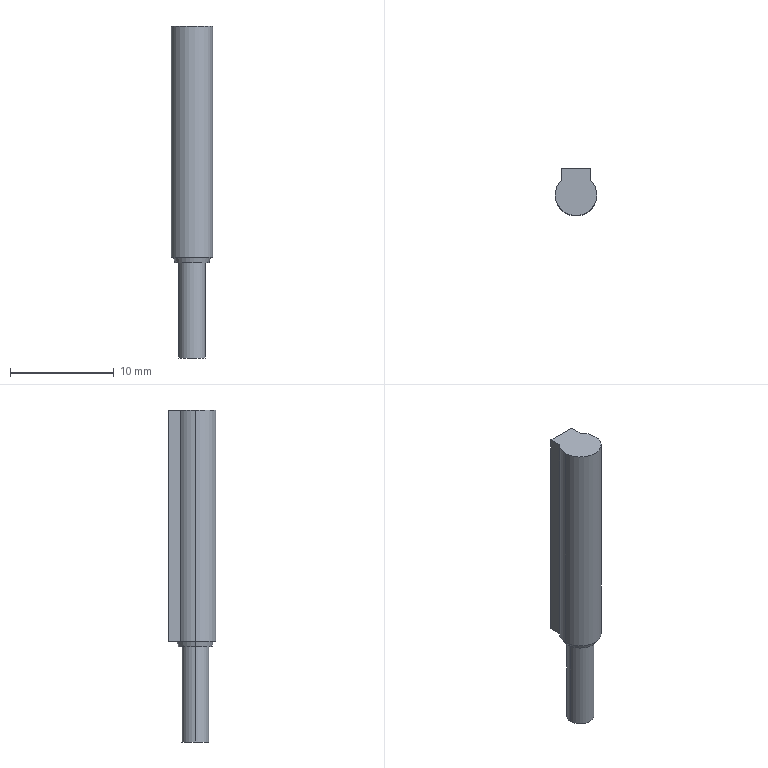Part | SolidWorks | features BaseBody 1 | 1 solid | 24 faces | box 4 x 4.6 x 32 mm | volume 381.799 mm3 | plane 12 | cylinder 10 | cone 2 | commonest cylinder face diameters 2.1 x3 4 x3 2.5 x2 2.6 x2
STEP:
#1=CARTESIAN_POINT('',(-1.4,1.428,-22.3));
#2=VERTEX_POINT('',#1);
#3=CARTESIAN_POINT('',(-2.,0.,-22.3));
#4=VERTEX_POINT('',#3);
#5=CARTESIAN_POINT('',(0.,0.,-22.3));
#6=DIRECTION('',(0.,0.,1.));
#7=DIRECTION('',(1.,0.,0.));
#8=AXIS2_PLACEMENT_3D('',#5,#6,#7);
#9=CIRCLE('',#8,2.);
#10=EDGE_CURVE('',#2,#4,#9,.T.);
#11=ORIENTED_EDGE('',*,*,#10,.T.);
#12=CARTESIAN_POINT('',(-2.,0.,0.));
#13=VERTEX_POINT('',#12);
#14=CARTESIAN_POINT('',(-2.,0.,-22.3));
#15=DIRECTION('',(0.,0.,1.));
#16=VECTOR('',#15,1000.);
#17=LINE('',#14,#16);
#18=EDGE_CURVE('',#4,#13,#17,.T.);
#19=ORIENTED_EDGE('',*,*,#18,.T.);
#20=CARTESIAN_POINT('',(-1.4,1.428,0.));
#21=VERTEX_POINT('',#20);
#22=CARTESIAN_POINT('',(0.,0.,0.));
#23=DIRECTION('',(0.,0.,-1.));
#24=DIRECTION('',(1.,0.,0.));
#25=AXIS2_PLACEMENT_3D('',#22,#23,#24);
#26=CIRCLE('',#25,2.);
#27=EDGE_CURVE('',#13,#21,#26,.T.);
#28=ORIENTED_EDGE('',*,*,#27,.T.);
#29=CARTESIAN_POINT('',(-1.4,1.428,-22.3));
#30=DIRECTION('',(0.,0.,-1.));
#31=VECTOR('',#30,1000.);
#32=LINE('',#29,#31);
#33=EDGE_CURVE('',#21,#2,#32,.T.);
#34=ORIENTED_EDGE('',*,*,#33,.T.);
#35=EDGE_LOOP('',(#11,#19,#28,#34));
#36=FACE_OUTER_BOUND('',#35,.T.);
#37=CARTESIAN_POINT('',(0.,0.,-22.3));
#38=DIRECTION('',(0.,0.,1.));
#39=DIRECTION('',(1.,0.,0.));
#40=AXIS2_PLACEMENT_3D('',#37,#38,#39);
#41=CYLINDRICAL_SURFACE('',#40,2.);
#42=ADVANCED_FACE('',(#36),#41,.T.);
#43=ORIENTED_EDGE('',*,*,#18,.F.);
#44=CARTESIAN_POINT('',(2.,0.,-22.3));
#45=VERTEX_POINT('',#44);
#46=CARTESIAN_POINT('',(0.,0.,-22.3));
#47=DIRECTION('',(0.,0.,1.));
#48=DIRECTION('',(1.,0.,0.));
#49=AXIS2_PLACEMENT_3D('',#46,#47,#48);
#50=CIRCLE('',#49,2.);
#51=EDGE_CURVE('',#4,#45,#50,.T.);
#52=ORIENTED_EDGE('',*,*,#51,.T.);
#53=CARTESIAN_POINT('',(2.,0.,0.));
#54=VERTEX_POINT('',#53);
#55=CARTESIAN_POINT('',(2.,0.,-22.3));
#56=DIRECTION('',(0.,0.,1.));
#57=VECTOR('',#56,1000.);
#58=LINE('',#55,#57);
#59=EDGE_CURVE('',#45,#54,#58,.T.);
#60=ORIENTED_EDGE('',*,*,#59,.T.);
#61=CARTESIAN_POINT('',(0.,0.,0.));
#62=DIRECTION('',(0.,0.,-1.));
#63=DIRECTION('',(1.,0.,0.));
#64=AXIS2_PLACEMENT_3D('',#61,#62,#63);
#65=CIRCLE('',#64,2.);
#66=EDGE_CURVE('',#54,#13,#65,.T.);
#67=ORIENTED_EDGE('',*,*,#66,.T.);
#68=EDGE_LOOP('',(#43,#52,#60,#67));
#69=FACE_OUTER_BOUND('',#68,.T.);
#70=CARTESIAN_POINT('',(0.,0.,-22.3));
#71=DIRECTION('',(0.,0.,1.));
#72=DIRECTION('',(1.,0.,0.));
#73=AXIS2_PLACEMENT_3D('',#70,#71,#72);
#74=CYLINDRICAL_SURFACE('',#73,2.);
#75=ADVANCED_FACE('',(#69),#74,.T.);
#76=CARTESIAN_POINT('',(1.65,0.,-22.8));
#77=VERTEX_POINT('',#76);
#78=CARTESIAN_POINT('',(-1.65,0.,-22.8));
#79=VERTEX_POINT('',#78);
#80=CARTESIAN_POINT('',(0.,0.,-22.8));
#81=DIRECTION('',(0.,0.,1.));
#82=DIRECTION('',(1.,0.,0.));
#83=AXIS2_PLACEMENT_3D('',#80,#81,#82);
#84=CIRCLE('',#83,1.65);
#85=EDGE_CURVE('',#77,#79,#84,.T.);
#86=ORIENTED_EDGE('',*,*,#85,.T.);
#87=CARTESIAN_POINT('',(-1.784,0.,-22.3));
#88=VERTEX_POINT('',#87);
#89=CARTESIAN_POINT('',(-1.784,0.,-22.3));
#90=DIRECTION('',(-0.2588,0.,0.9659));
#91=VECTOR('',#90,1000.);
#92=LINE('',#89,#91);
#93=EDGE_CURVE('',#79,#88,#92,.T.);
#94=ORIENTED_EDGE('',*,*,#93,.T.);
#95=CARTESIAN_POINT('',(1.784,0.,-22.3));
#96=VERTEX_POINT('',#95);
#97=CARTESIAN_POINT('',(0.,0.,-22.3));
#98=DIRECTION('',(0.,0.,-1.));
#99=DIRECTION('',(1.,0.,0.));
#100=AXIS2_PLACEMENT_3D('',#97,#98,#99);
#101=CIRCLE('',#100,1.784);
#102=EDGE_CURVE('',#88,#96,#101,.T.);
#103=ORIENTED_EDGE('',*,*,#102,.T.);
#104=CARTESIAN_POINT('',(1.784,0.,-22.3));
#105=DIRECTION('',(0.2588,0.,0.9659));
#106=VECTOR('',#105,1000.);
#107=LINE('',#104,#106);
#108=EDGE_CURVE('',#77,#96,#107,.T.);
#109=ORIENTED_EDGE('',*,*,#108,.F.);
#110=EDGE_LOOP('',(#86,#94,#103,#109));
#111=FACE_OUTER_BOUND('',#110,.T.);
#112=CARTESIAN_POINT('',(0.,0.,-22.3));
#113=DIRECTION('',(0.,0.,1.));
#114=DIRECTION('',(1.,0.,0.));
#115=AXIS2_PLACEMENT_3D('',#112,#113,#114);
#116=CONICAL_SURFACE('',#115,1.784,0.2618);
#117=ADVANCED_FACE('',(#111),#116,.T.);
#118=CARTESIAN_POINT('',(0.,2.4,-3.25));
#119=VERTEX_POINT('',#118);
#120=CARTESIAN_POINT('',(0.,2.4,-0.75));
#121=VERTEX_POINT('',#120);
#122=CARTESIAN_POINT('',(0.,2.4,-2.));
#123=DIRECTION('',(0.,1.,0.));
#124=DIRECTION('',(0.,0.,1.));
#125=AXIS2_PLACEMENT_3D('',#122,#123,#124);
#126=CIRCLE('',#125,1.25);
#127=EDGE_CURVE('',#119,#121,#126,.T.);
#128=ORIENTED_EDGE('',*,*,#127,.F.);
#129=CARTESIAN_POINT('',(0.,2.6,-3.25));
#130=VERTEX_POINT('',#129);
#131=CARTESIAN_POINT('',(0.,2.4,-3.25));
#132=DIRECTION('',(0.,1.,0.));
#133=VECTOR('',#132,1000.);
#134=LINE('',#131,#133);
#135=EDGE_CURVE('',#119,#130,#134,.T.);
#136=ORIENTED_EDGE('',*,*,#135,.T.);
#137=CARTESIAN_POINT('',(0.,2.6,-0.75));
#138=VERTEX_POINT('',#137);
#139=CARTESIAN_POINT('',(0.,2.6,-2.));
#140=DIRECTION('',(0.,-1.,0.));
#141=DIRECTION('',(0.,0.,1.));
#142=AXIS2_PLACEMENT_3D('',#139,#140,#141);
#143=CIRCLE('',#142,1.25);
#144=EDGE_CURVE('',#138,#130,#143,.T.);
#145=ORIENTED_EDGE('',*,*,#144,.F.);
#146=CARTESIAN_POINT('',(0.,2.4,-0.75));
#147=DIRECTION('',(0.,1.,0.));
#148=VECTOR('',#147,1000.);
#149=LINE('',#146,#148);
#150=EDGE_CURVE('',#121,#138,#149,.T.);
#151=ORIENTED_EDGE('',*,*,#150,.F.);
#152=EDGE_LOOP('',(#128,#136,#145,#151));
#153=FACE_OUTER_BOUND('',#152,.T.);
#154=CARTESIAN_POINT('',(0.,2.4,-2.));
#155=DIRECTION('',(0.,1.,0.));
#156=DIRECTION('',(0.,0.,1.));
#157=AXIS2_PLACEMENT_3D('',#154,#155,#156);
#158=CYLINDRICAL_SURFACE('',#157,1.25);
#159=ADVANCED_FACE('',(#153),#158,.F.);
#160=CARTESIAN_POINT('',(1.3,0.,-32.));
#161=VERTEX_POINT('',#160);
#162=CARTESIAN_POINT('',(-1.3,0.,-32.));
#163=VERTEX_POINT('',#162);
#164=CARTESIAN_POINT('',(0.,0.,-32.));
#165=DIRECTION('',(0.,0.,1.));
#166=DIRECTION('',(1.,0.,0.));
#167=AXIS2_PLACEMENT_3D('',#164,#165,#166);
#168=CIRCLE('',#167,1.3);
#169=EDGE_CURVE('',#161,#163,#168,.T.);
#170=ORIENTED_EDGE('',*,*,#169,.T.);
#171=CARTESIAN_POINT('',(-1.3,0.,-22.8));
#172=VERTEX_POINT('',#171);
#173=CARTESIAN_POINT('',(-1.3,0.,-32.));
#174=DIRECTION('',(0.,0.,1.));
#175=VECTOR('',#174,1000.);
#176=LINE('',#173,#175);
#177=EDGE_CURVE('',#163,#172,#176,.T.);
#178=ORIENTED_EDGE('',*,*,#177,.T.);
#179=CARTESIAN_POINT('',(1.3,0.,-22.8));
#180=VERTEX_POINT('',#179);
#181=CARTESIAN_POINT('',(0.,0.,-22.8));
#182=DIRECTION('',(0.,0.,-1.));
#183=DIRECTION('',(1.,0.,0.));
#184=AXIS2_PLACEMENT_3D('',#181,#182,#183);
#185=CIRCLE('',#184,1.3);
#186=EDGE_CURVE('',#172,#180,#185,.T.);
#187=ORIENTED_EDGE('',*,*,#186,.T.);
#188=CARTESIAN_POINT('',(1.3,0.,-32.));
#189=DIRECTION('',(0.,0.,1.));
#190=VECTOR('',#189,1000.);
#191=LINE('',#188,#190);
#192=EDGE_CURVE('',#161,#180,#191,.T.);
#193=ORIENTED_EDGE('',*,*,#192,.F.);
#194=EDGE_LOOP('',(#170,#178,#187,#193));
#195=FACE_OUTER_BOUND('',#194,.T.);
#196=CARTESIAN_POINT('',(0.,0.,-32.));
#197=DIRECTION('',(0.,0.,1.));
#198=DIRECTION('',(1.,0.,0.));
#199=AXIS2_PLACEMENT_3D('',#196,#197,#198);
#200=CYLINDRICAL_SURFACE('',#199,1.3);
#201=ADVANCED_FACE('',(#195),#200,.T.);
#202=CARTESIAN_POINT('',(0.,2.4,-0.95));
#203=VERTEX_POINT('',#202);
#204=CARTESIAN_POINT('',(-0.5443,2.4,-1.102));
#205=VERTEX_POINT('',#204);
#206=CARTESIAN_POINT('',(0.,2.4,-2.));
#207=DIRECTION('',(0.,-1.,0.));
#208=DIRECTION('',(0.,0.,1.));
#209=AXIS2_PLACEMENT_3D('',#206,#207,#208);
#210=CIRCLE('',#209,1.05);
#211=EDGE_CURVE('',#203,#205,#210,.T.);
#212=ORIENTED_EDGE('',*,*,#211,.F.);
#213=CARTESIAN_POINT('',(0.,2.6,-0.95));
#214=VERTEX_POINT('',#213);
#215=CARTESIAN_POINT('',(0.,2.4,-0.95));
#216=DIRECTION('',(0.,1.,0.));
#217=VECTOR('',#216,1000.);
#218=LINE('',#215,#217);
#219=EDGE_CURVE('',#203,#214,#218,.T.);
#220=ORIENTED_EDGE('',*,*,#219,.T.);
#221=CARTESIAN_POINT('',(-0.5443,2.6,-1.102));
#222=VERTEX_POINT('',#221);
#223=CARTESIAN_POINT('',(0.,2.6,-2.));
#224=DIRECTION('',(0.,-1.,0.));
#225=DIRECTION('',(0.,0.,1.));
#226=AXIS2_PLACEMENT_3D('',#223,#224,#225);
#227=CIRCLE('',#226,1.05);
#228=EDGE_CURVE('',#214,#222,#227,.T.);
#229=ORIENTED_EDGE('',*,*,#228,.T.);
#230=CARTESIAN_POINT('',(-0.5443,2.4,-1.102));
#231=DIRECTION('',(0.,-1.,0.));
#232=VECTOR('',#231,1000.);
#233=LINE('',#230,#232);
#234=EDGE_CURVE('',#222,#205,#233,.T.);
#235=ORIENTED_EDGE('',*,*,#234,.T.);
#236=EDGE_LOOP('',(#212,#220,#229,#235));
#237=FACE_OUTER_BOUND('',#236,.T.);
#238=CARTESIAN_POINT('',(0.,2.4,-2.));
#239=DIRECTION('',(0.,1.,0.));
#240=DIRECTION('',(0.,0.,1.));
#241=AXIS2_PLACEMENT_3D('',#238,#239,#240);
#242=CYLINDRICAL_SURFACE('',#241,1.05);
#243=ADVANCED_FACE('',(#237),#242,.T.);
#244=ORIENTED_EDGE('',*,*,#59,.F.);
#245=CARTESIAN_POINT('',(1.4,1.428,-22.3));
#246=VERTEX_POINT('',#245);
#247=CARTESIAN_POINT('',(0.,0.,-22.3));
#248=DIRECTION('',(0.,0.,1.));
#249=DIRECTION('',(1.,0.,0.));
#250=AXIS2_PLACEMENT_3D('',#247,#248,#249);
#251=CIRCLE('',#250,2.);
#252=EDGE_CURVE('',#45,#246,#251,.T.);
#253=ORIENTED_EDGE('',*,*,#252,.T.);
#254=CARTESIAN_POINT('',(1.4,1.428,0.));
#255=VERTEX_POINT('',#254);
#256=CARTESIAN_POINT('',(1.4,1.428,-22.3));
#257=DIRECTION('',(0.,0.,1.));
#258=VECTOR('',#257,1000.);
#259=LINE('',#256,#258);
#260=EDGE_CURVE('',#246,#255,#259,.T.);
#261=ORIENTED_EDGE('',*,*,#260,.T.);
#262=CARTESIAN_POINT('',(0.,0.,0.));
#263=DIRECTION('',(0.,0.,-1.));
#264=DIRECTION('',(1.,0.,0.));
#265=AXIS2_PLACEMENT_3D('',#262,#263,#264);
#266=CIRCLE('',#265,2.);
#267=EDGE_CURVE('',#255,#54,#266,.T.);
#268=ORIENTED_EDGE('',*,*,#267,.T.);
#269=EDGE_LOOP('',(#244,#253,#261,#268));
#270=FACE_OUTER_BOUND('',#269,.T.);
#271=CARTESIAN_POINT('',(0.,0.,-22.3));
#272=DIRECTION('',(0.,0.,1.));
#273=DIRECTION('',(1.,0.,0.));
#274=AXIS2_PLACEMENT_3D('',#271,#272,#273);
#275=CYLINDRICAL_SURFACE('',#274,2.);
#276=ADVANCED_FACE('',(#270),#275,.T.);
#277=CARTESIAN_POINT('',(1.4,2.6,-22.3));
#278=VERTEX_POINT('',#277);
#279=CARTESIAN_POINT('',(1.4,1.428,-22.3));
#280=DIRECTION('',(0.,1.,0.));
#281=VECTOR('',#280,1000.);
#282=LINE('',#279,#281);
#283=EDGE_CURVE('',#246,#278,#282,.T.);
#284=ORIENTED_EDGE('',*,*,#283,.T.);
#285=CARTESIAN_POINT('',(1.4,2.6,0.));
#286=VERTEX_POINT('',#285);
#287=CARTESIAN_POINT('',(1.4,2.6,-22.3));
#288=DIRECTION('',(0.,0.,1.));
#289=VECTOR('',#288,1000.);
#290=LINE('',#287,#289);
#291=EDGE_CURVE('',#278,#286,#290,.T.);
#292=ORIENTED_EDGE('',*,*,#291,.T.);
#293=CARTESIAN_POINT('',(1.4,1.428,0.));
#294=DIRECTION('',(0.,-1.,0.));
#295=VECTOR('',#294,1000.);
#296=LINE('',#293,#295);
#297=EDGE_CURVE('',#286,#255,#296,.T.);
#298=ORIENTED_EDGE('',*,*,#297,.T.);
#299=ORIENTED_EDGE('',*,*,#260,.F.);
#300=EDGE_LOOP('',(#284,#292,#298,#299));
#301=FACE_OUTER_BOUND('',#300,.T.);
#302=CARTESIAN_POINT('',(1.4,1.428,-22.3));
#303=DIRECTION('',(1.,0.,0.));
#304=DIRECTION('',(0.,1.,0.));
#305=AXIS2_PLACEMENT_3D('',#302,#303,#304);
#306=PLANE('',#305);
#307=ADVANCED_FACE('',(#301),#306,.T.);
#308=CARTESIAN_POINT('',(-1.4,2.6,-22.3));
#309=VERTEX_POINT('',#308);
#310=CARTESIAN_POINT('',(0.,2.6,-22.3));
#311=DIRECTION('',(-1.,0.,0.));
#312=VECTOR('',#311,1000.);
#313=LINE('',#310,#312);
#314=EDGE_CURVE('',#278,#309,#313,.T.);
#315=ORIENTED_EDGE('',*,*,#314,.F.);
#316=ORIENTED_EDGE('',*,*,#283,.F.);
#317=ORIENTED_EDGE('',*,*,#252,.F.);
#318=ORIENTED_EDGE('',*,*,#51,.F.);
#319=ORIENTED_EDGE('',*,*,#10,.F.);
#320=CARTESIAN_POINT('',(-1.4,0.,-22.3));
#321=DIRECTION('',(0.,-1.,0.));
#322=VECTOR('',#321,1000.);
#323=LINE('',#320,#322);
#324=EDGE_CURVE('',#309,#2,#323,.T.);
#325=ORIENTED_EDGE('',*,*,#324,.F.);
#326=EDGE_LOOP('',(#315,#316,#317,#318,#319,#325));
#327=FACE_OUTER_BOUND('',#326,.T.);
#328=CARTESIAN_POINT('',(0.,0.,-22.3));
#329=DIRECTION('',(0.,0.,-1.));
#330=DIRECTION('',(1.,0.,0.));
#331=AXIS2_PLACEMENT_3D('',#328,#329,#330);
#332=CIRCLE('',#331,1.784);
#333=EDGE_CURVE('',#96,#88,#332,.T.);
#334=ORIENTED_EDGE('',*,*,#333,.F.);
#335=ORIENTED_EDGE('',*,*,#102,.F.);
#336=EDGE_LOOP('',(#334,#335));
#337=FACE_BOUND('',#336,.T.);
#338=CARTESIAN_POINT('',(0.,0.,-22.3));
#339=DIRECTION('',(0.,0.,1.));
#340=DIRECTION('',(1.,0.,0.));
#341=AXIS2_PLACEMENT_3D('',#338,#339,#340);
#342=PLANE('',#341);
#343=ADVANCED_FACE('',(#327,#337),#342,.F.);
#344=ORIENTED_EDGE('',*,*,#324,.T.);
#345=ORIENTED_EDGE('',*,*,#33,.F.);
#346=CARTESIAN_POINT('',(-1.4,2.6,0.));
#347=VERTEX_POINT('',#346);
#348=CARTESIAN_POINT('',(-1.4,2.6,0.));
#349=DIRECTION('',(0.,1.,0.));
#350=VECTOR('',#349,1000.);
#351=LINE('',#348,#350);
#352=EDGE_CURVE('',#21,#347,#351,.T.);
#353=ORIENTED_EDGE('',*,*,#352,.T.);
#354=CARTESIAN_POINT('',(-1.4,2.6,-22.3));
#355=DIRECTION('',(0.,0.,-1.));
#356=VECTOR('',#355,1000.);
#357=LINE('',#354,#356);
#358=EDGE_CURVE('',#347,#309,#357,.T.);
#359=ORIENTED_EDGE('',*,*,#358,.T.);
#360=EDGE_LOOP('',(#344,#345,#353,#359));
#361=FACE_OUTER_BOUND('',#360,.T.);
#362=CARTESIAN_POINT('',(-1.4,2.6,-22.3));
#363=DIRECTION('',(-1.,0.,0.));
#364=DIRECTION('',(0.,-1.,0.));
#365=AXIS2_PLACEMENT_3D('',#362,#363,#364);
#366=PLANE('',#365);
#367=ADVANCED_FACE('',(#361),#366,.T.);
#368=ORIENTED_EDGE('',*,*,#297,.F.);
#369=CARTESIAN_POINT('',(0.,2.6,0.));
#370=DIRECTION('',(-1.,0.,0.));
#371=VECTOR('',#370,1000.);
#372=LINE('',#369,#371);
#373=EDGE_CURVE('',#286,#347,#372,.T.);
#374=ORIENTED_EDGE('',*,*,#373,.T.);
#375=ORIENTED_EDGE('',*,*,#352,.F.);
#376=ORIENTED_EDGE('',*,*,#27,.F.);
#377=ORIENTED_EDGE('',*,*,#66,.F.);
#378=ORIENTED_EDGE('',*,*,#267,.F.);
#379=EDGE_LOOP('',(#368,#374,#375,#376,#377,#378));
#380=FACE_OUTER_BOUND('',#379,.T.);
#381=CARTESIAN_POINT('',(0.,0.,0.));
#382=DIRECTION('',(0.,0.,1.));
#383=DIRECTION('',(1.,0.,0.));
#384=AXIS2_PLACEMENT_3D('',#381,#382,#383);
#385=PLANE('',#384);
#386=ADVANCED_FACE('',(#380),#385,.T.);
#387=ORIENTED_EDGE('',*,*,#314,.T.);
#388=ORIENTED_EDGE('',*,*,#358,.F.);
#389=ORIENTED_EDGE('',*,*,#373,.F.);
#390=ORIENTED_EDGE('',*,*,#291,.F.);
#391=EDGE_LOOP('',(#387,#388,#389,#390));
#392=FACE_OUTER_BOUND('',#391,.T.);
#393=ORIENTED_EDGE('',*,*,#144,.T.);
#394=CARTESIAN_POINT('',(0.,2.6,-2.));
#395=DIRECTION('',(0.,-1.,0.));
#396=DIRECTION('',(0.,0.,1.));
#397=AXIS2_PLACEMENT_3D('',#394,#395,#396);
#398=CIRCLE('',#397,1.25);
#399=EDGE_CURVE('',#130,#138,#398,.T.);
#400=ORIENTED_EDGE('',*,*,#399,.T.);
#401=EDGE_LOOP('',(#393,#400));
#402=FACE_BOUND('',#401,.T.);
#403=CARTESIAN_POINT('',(1.4,2.6,-22.3));
#404=DIRECTION('',(0.,1.,0.));
#405=DIRECTION('',(0.,0.,1.));
#406=AXIS2_PLACEMENT_3D('',#403,#404,#405);
#407=PLANE('',#406);
#408=ADVANCED_FACE('',(#392,#402),#407,.T.);
#409=ORIENTED_EDGE('',*,*,#93,.F.);
#410=CARTESIAN_POINT('',(0.,0.,-22.8));
#411=DIRECTION('',(0.,0.,1.));
#412=DIRECTION('',(1.,0.,0.));
#413=AXIS2_PLACEMENT_3D('',#410,#411,#412);
#414=CIRCLE('',#413,1.65);
#415=EDGE_CURVE('',#79,#77,#414,.T.);
#416=ORIENTED_EDGE('',*,*,#415,.T.);
#417=ORIENTED_EDGE('',*,*,#108,.T.);
#418=ORIENTED_EDGE('',*,*,#333,.T.);
#419=EDGE_LOOP('',(#409,#416,#417,#418));
#420=FACE_OUTER_BOUND('',#419,.T.);
#421=CARTESIAN_POINT('',(0.,0.,-22.3));
#422=DIRECTION('',(0.,0.,1.));
#423=DIRECTION('',(1.,0.,0.));
#424=AXIS2_PLACEMENT_3D('',#421,#422,#423);
#425=CONICAL_SURFACE('',#424,1.784,0.2618);
#426=ADVANCED_FACE('',(#420),#425,.T.);
#427=ORIENTED_EDGE('',*,*,#135,.F.);
#428=CARTESIAN_POINT('',(0.,2.4,-2.));
#429=DIRECTION('',(0.,1.,0.));
#430=DIRECTION('',(0.,0.,1.));
#431=AXIS2_PLACEMENT_3D('',#428,#429,#430);
#432=CIRCLE('',#431,1.25);
#433=EDGE_CURVE('',#121,#119,#432,.T.);
#434=ORIENTED_EDGE('',*,*,#433,.F.);
#435=ORIENTED_EDGE('',*,*,#150,.T.);
#436=ORIENTED_EDGE('',*,*,#399,.F.);
#437=EDGE_LOOP('',(#427,#434,#435,#436));
#438=FACE_OUTER_BOUND('',#437,.T.);
#439=CARTESIAN_POINT('',(0.,2.4,-2.));
#440=DIRECTION('',(0.,1.,0.));
#441=DIRECTION('',(0.,0.,1.));
#442=AXIS2_PLACEMENT_3D('',#439,#440,#441);
#443=CYLINDRICAL_SURFACE('',#442,1.25);
#444=ADVANCED_FACE('',(#438),#443,.F.);
#445=ORIENTED_EDGE('',*,*,#85,.F.);
#446=ORIENTED_EDGE('',*,*,#415,.F.);
#447=EDGE_LOOP('',(#445,#446));
#448=FACE_OUTER_BOUND('',#447,.T.);
#449=CARTESIAN_POINT('',(0.,0.,-22.8));
#450=DIRECTION('',(0.,0.,-1.));
#451=DIRECTION('',(1.,0.,0.));
#452=AXIS2_PLACEMENT_3D('',#449,#450,#451);
#453=CIRCLE('',#452,1.3);
#454=EDGE_CURVE('',#180,#172,#453,.T.);
#455=ORIENTED_EDGE('',*,*,#454,.F.);
#456=ORIENTED_EDGE('',*,*,#186,.F.);
#457=EDGE_LOOP('',(#455,#456));
#458=FACE_BOUND('',#457,.T.);
#459=CARTESIAN_POINT('',(0.,1.65,-22.8));
#460=DIRECTION('',(0.,0.,1.));
#461=DIRECTION('',(1.,0.,0.));
#462=AXIS2_PLACEMENT_3D('',#459,#460,#461);
#463=PLANE('',#462);
#464=ADVANCED_FACE('',(#448,#458),#463,.F.);
#465=ORIENTED_EDGE('',*,*,#433,.T.);
#466=ORIENTED_EDGE('',*,*,#127,.T.);
#467=EDGE_LOOP('',(#465,#466));
#468=FACE_OUTER_BOUND('',#467,.T.);
#469=CARTESIAN_POINT('',(0.8979,2.4,-2.544));
#470=VERTEX_POINT('',#469);
#471=CARTESIAN_POINT('',(-0.5443,2.4,-1.102));
#472=DIRECTION('',(0.7071,0.,-0.7071));
#473=VECTOR('',#472,1000.);
#474=LINE('',#471,#473);
#475=EDGE_CURVE('',#205,#470,#474,.T.);
#476=ORIENTED_EDGE('',*,*,#475,.T.);
#477=CARTESIAN_POINT('',(0.,2.4,-2.));
#478=DIRECTION('',(0.,-1.,0.));
#479=DIRECTION('',(0.,0.,1.));
#480=AXIS2_PLACEMENT_3D('',#477,#478,#479);
#481=CIRCLE('',#480,1.05);
#482=EDGE_CURVE('',#470,#203,#481,.T.);
#483=ORIENTED_EDGE('',*,*,#482,.T.);
#484=ORIENTED_EDGE('',*,*,#211,.T.);
#485=EDGE_LOOP('',(#476,#483,#484));
#486=FACE_BOUND('',#485,.T.);
#487=CARTESIAN_POINT('',(0.5443,2.4,-2.898));
#488=VERTEX_POINT('',#487);
#489=CARTESIAN_POINT('',(-0.8979,2.4,-1.456));
#490=VERTEX_POINT('',#489);
#491=CARTESIAN_POINT('',(0.5443,2.4,-2.898));
#492=DIRECTION('',(-0.7071,0.,0.7071));
#493=VECTOR('',#492,1000.);
#494=LINE('',#491,#493);
#495=EDGE_CURVE('',#488,#490,#494,.T.);
#496=ORIENTED_EDGE('',*,*,#495,.T.);
#497=CARTESIAN_POINT('',(0.,2.4,-2.));
#498=DIRECTION('',(0.,-1.,0.));
#499=DIRECTION('',(0.,0.,1.));
#500=AXIS2_PLACEMENT_3D('',#497,#498,#499);
#501=CIRCLE('',#500,1.05);
#502=EDGE_CURVE('',#490,#488,#501,.T.);
#503=ORIENTED_EDGE('',*,*,#502,.T.);
#504=EDGE_LOOP('',(#496,#503));
#505=FACE_BOUND('',#504,.T.);
#506=CARTESIAN_POINT('',(0.,2.4,-2.));
#507=DIRECTION('',(0.,1.,0.));
#508=DIRECTION('',(0.,0.,1.));
#509=AXIS2_PLACEMENT_3D('',#506,#507,#508);
#510=PLANE('',#509);
#511=ADVANCED_FACE('',(#468,#486,#505),#510,.T.);
#512=ORIENTED_EDGE('',*,*,#177,.F.);
#513=CARTESIAN_POINT('',(0.,0.,-32.));
#514=DIRECTION('',(0.,0.,1.));
#515=DIRECTION('',(1.,0.,0.));
#516=AXIS2_PLACEMENT_3D('',#513,#514,#515);
#517=CIRCLE('',#516,1.3);
#518=EDGE_CURVE('',#163,#161,#517,.T.);
#519=ORIENTED_EDGE('',*,*,#518,.T.);
#520=ORIENTED_EDGE('',*,*,#192,.T.);
#521=ORIENTED_EDGE('',*,*,#454,.T.);
#522=EDGE_LOOP('',(#512,#519,#520,#521));
#523=FACE_OUTER_BOUND('',#522,.T.);
#524=CARTESIAN_POINT('',(0.,0.,-32.));
#525=DIRECTION('',(0.,0.,1.));
#526=DIRECTION('',(1.,0.,0.));
#527=AXIS2_PLACEMENT_3D('',#524,#525,#526);
#528=CYLINDRICAL_SURFACE('',#527,1.3);
#529=ADVANCED_FACE('',(#523),#528,.T.);
#530=ORIENTED_EDGE('',*,*,#219,.F.);
#531=ORIENTED_EDGE('',*,*,#482,.F.);
#532=CARTESIAN_POINT('',(0.8979,2.6,-2.544));
#533=VERTEX_POINT('',#532);
#534=CARTESIAN_POINT('',(0.8979,2.4,-2.544));
#535=DIRECTION('',(0.,1.,0.));
#536=VECTOR('',#535,1000.);
#537=LINE('',#534,#536);
#538=EDGE_CURVE('',#470,#533,#537,.T.);
#539=ORIENTED_EDGE('',*,*,#538,.T.);
#540=CARTESIAN_POINT('',(0.,2.6,-2.));
#541=DIRECTION('',(0.,-1.,0.));
#542=DIRECTION('',(0.,0.,1.));
#543=AXIS2_PLACEMENT_3D('',#540,#541,#542);
#544=CIRCLE('',#543,1.05);
#545=EDGE_CURVE('',#533,#214,#544,.T.);
#546=ORIENTED_EDGE('',*,*,#545,.T.);
#547=EDGE_LOOP('',(#530,#531,#539,#546));
#548=FACE_OUTER_BOUND('',#547,.T.);
#549=CARTESIAN_POINT('',(0.,2.4,-2.));
#550=DIRECTION('',(0.,1.,0.));
#551=DIRECTION('',(0.,0.,1.));
#552=AXIS2_PLACEMENT_3D('',#549,#550,#551);
#553=CYLINDRICAL_SURFACE('',#552,1.05);
#554=ADVANCED_FACE('',(#548),#553,.T.);
#555=ORIENTED_EDGE('',*,*,#475,.F.);
#556=ORIENTED_EDGE('',*,*,#234,.F.);
#557=CARTESIAN_POINT('',(0.8979,2.6,-2.544));
#558=DIRECTION('',(0.7071,0.,-0.7071));
#559=VECTOR('',#558,1000.);
#560=LINE('',#557,#559);
#561=EDGE_CURVE('',#222,#533,#560,.T.);
#562=ORIENTED_EDGE('',*,*,#561,.T.);
#563=ORIENTED_EDGE('',*,*,#538,.F.);
#564=EDGE_LOOP('',(#555,#556,#562,#563));
#565=FACE_OUTER_BOUND('',#564,.T.);
#566=CARTESIAN_POINT('',(0.8979,2.4,-2.544));
#567=DIRECTION('',(-0.7071,0.,-0.7071));
#568=DIRECTION('',(-0.7071,0.,0.7071));
#569=AXIS2_PLACEMENT_3D('',#566,#567,#568);
#570=PLANE('',#569);
#571=ADVANCED_FACE('',(#565),#570,.T.);
#572=ORIENTED_EDGE('',*,*,#502,.F.);
#573=CARTESIAN_POINT('',(-0.8979,2.6,-1.456));
#574=VERTEX_POINT('',#573);
#575=CARTESIAN_POINT('',(-0.8979,2.4,-1.456));
#576=DIRECTION('',(0.,1.,0.));
#577=VECTOR('',#576,1000.);
#578=LINE('',#575,#577);
#579=EDGE_CURVE('',#490,#574,#578,.T.);
#580=ORIENTED_EDGE('',*,*,#579,.T.);
#581=CARTESIAN_POINT('',(0.5443,2.6,-2.898));
#582=VERTEX_POINT('',#581);
#583=CARTESIAN_POINT('',(0.,2.6,-2.));
#584=DIRECTION('',(0.,-1.,0.));
#585=DIRECTION('',(0.,0.,1.));
#586=AXIS2_PLACEMENT_3D('',#583,#584,#585);
#587=CIRCLE('',#586,1.05);
#588=EDGE_CURVE('',#574,#582,#587,.T.);
#589=ORIENTED_EDGE('',*,*,#588,.T.);
#590=CARTESIAN_POINT('',(0.5443,2.4,-2.898));
#591=DIRECTION('',(0.,-1.,0.));
#592=VECTOR('',#591,1000.);
#593=LINE('',#590,#592);
#594=EDGE_CURVE('',#582,#488,#593,.T.);
#595=ORIENTED_EDGE('',*,*,#594,.T.);
#596=EDGE_LOOP('',(#572,#580,#589,#595));
#597=FACE_OUTER_BOUND('',#596,.T.);
#598=CARTESIAN_POINT('',(0.,2.4,-2.));
#599=DIRECTION('',(0.,1.,0.));
#600=DIRECTION('',(0.,0.,1.));
#601=AXIS2_PLACEMENT_3D('',#598,#599,#600);
#602=CYLINDRICAL_SURFACE('',#601,1.05);
#603=ADVANCED_FACE('',(#597),#602,.T.);
#604=ORIENTED_EDGE('',*,*,#495,.F.);
#605=ORIENTED_EDGE('',*,*,#594,.F.);
#606=CARTESIAN_POINT('',(-0.8979,2.6,-1.456));
#607=DIRECTION('',(-0.7071,0.,0.7071));
#608=VECTOR('',#607,1000.);
#609=LINE('',#606,#608);
#610=EDGE_CURVE('',#582,#574,#609,.T.);
#611=ORIENTED_EDGE('',*,*,#610,.T.);
#612=ORIENTED_EDGE('',*,*,#579,.F.);
#613=EDGE_LOOP('',(#604,#605,#611,#612));
#614=FACE_OUTER_BOUND('',#613,.T.);
#615=CARTESIAN_POINT('',(-0.8979,2.4,-1.456));
#616=DIRECTION('',(0.7071,0.,0.7071));
#617=DIRECTION('',(0.7071,0.,-0.7071));
#618=AXIS2_PLACEMENT_3D('',#615,#616,#617);
#619=PLANE('',#618);
#620=ADVANCED_FACE('',(#614),#619,.T.);
#621=ORIENTED_EDGE('',*,*,#169,.F.);
#622=ORIENTED_EDGE('',*,*,#518,.F.);
#623=EDGE_LOOP('',(#621,#622));
#624=FACE_OUTER_BOUND('',#623,.T.);
#625=CARTESIAN_POINT('',(0.,0.,-32.));
#626=DIRECTION('',(0.,0.,1.));
#627=DIRECTION('',(1.,0.,0.));
#628=AXIS2_PLACEMENT_3D('',#625,#626,#627);
#629=PLANE('',#628);
#630=ADVANCED_FACE('',(#624),#629,.F.);
#631=ORIENTED_EDGE('',*,*,#545,.F.);
#632=ORIENTED_EDGE('',*,*,#561,.F.);
#633=ORIENTED_EDGE('',*,*,#228,.F.);
#634=EDGE_LOOP('',(#631,#632,#633));
#635=FACE_OUTER_BOUND('',#634,.T.);
#636=CARTESIAN_POINT('',(1.4,2.6,-22.3));
#637=DIRECTION('',(0.,1.,0.));
#638=DIRECTION('',(0.,0.,1.));
#639=AXIS2_PLACEMENT_3D('',#636,#637,#638);
#640=PLANE('',#639);
#641=ADVANCED_FACE('',(#635),#640,.T.);
#642=ORIENTED_EDGE('',*,*,#588,.F.);
#643=ORIENTED_EDGE('',*,*,#610,.F.);
#644=EDGE_LOOP('',(#642,#643));
#645=FACE_OUTER_BOUND('',#644,.T.);
#646=CARTESIAN_POINT('',(1.4,2.6,-22.3));
#647=DIRECTION('',(0.,1.,0.));
#648=DIRECTION('',(0.,0.,1.));
#649=AXIS2_PLACEMENT_3D('',#646,#647,#648);
#650=PLANE('',#649);
#651=ADVANCED_FACE('',(#645),#650,.T.);
#652=CLOSED_SHELL('',(#42,#75,#117,#159,#201,#243,#276,#307,#343,#367,#386,#408,#426,#444,#464,#511,#529,#554,#571,#603,#620,#630,#641,#651));
#653=MANIFOLD_SOLID_BREP('',#652);
#654=CARTESIAN_POINT('',(0.,0.,0.));
#655=DIRECTION('',(0.,0.,1.));
#656=DIRECTION('',(1.,0.,0.));
#657=AXIS2_PLACEMENT_3D('',#654,#655,#656);
#658=(LENGTH_UNIT()NAMED_UNIT(*)SI_UNIT(.MILLI.,.METRE.));
#659=UNCERTAINTY_MEASURE_WITH_UNIT(LENGTH_MEASURE(0.00001),#658,'','');
#660=(NAMED_UNIT(*)PLANE_ANGLE_UNIT()SI_UNIT($,.RADIAN.));
#661=(NAMED_UNIT(*)SI_UNIT($,.STERADIAN.)SOLID_ANGLE_UNIT());
#662=(GEOMETRIC_REPRESENTATION_CONTEXT(3)GLOBAL_UNCERTAINTY_ASSIGNED_CONTEXT((#659))GLOBAL_UNIT_ASSIGNED_CONTEXT((#658,#660,#661))REPRESENTATION_CONTEXT('',''));
#663=ADVANCED_BREP_SHAPE_REPRESENTATION('',(#653,#657),#662);